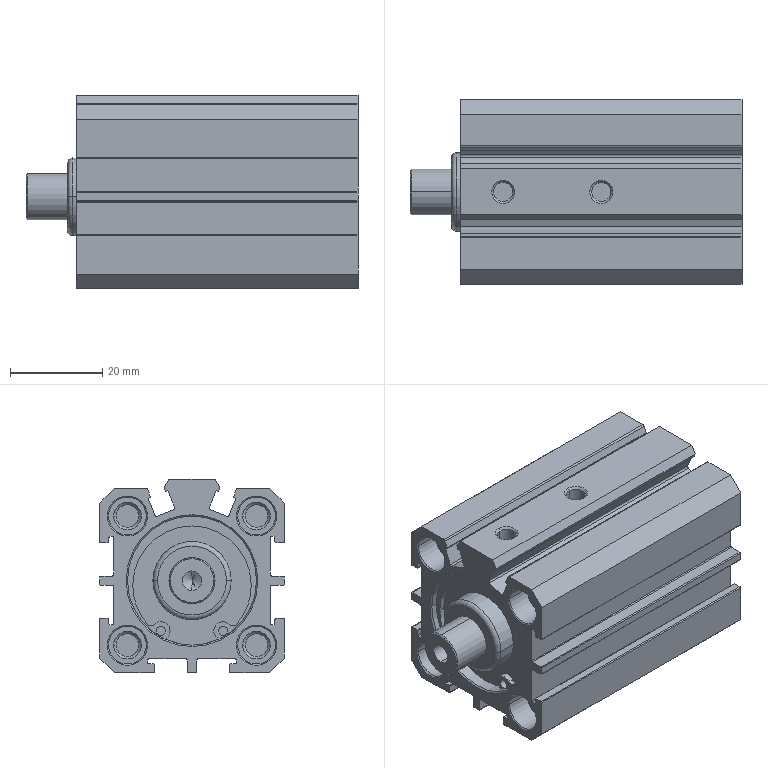Part | SolidWorks | 2 solids | 274 faces | box 72 x 40 x 42 mm | volume 66610 mm3 | cylinder 119 | plane 95 | cone 50 | torus 10 | commonest cylinder face diameters 0.4 x46 8.2 x16 4.917 x8 0.8 x7 2 x6 4.134 x4